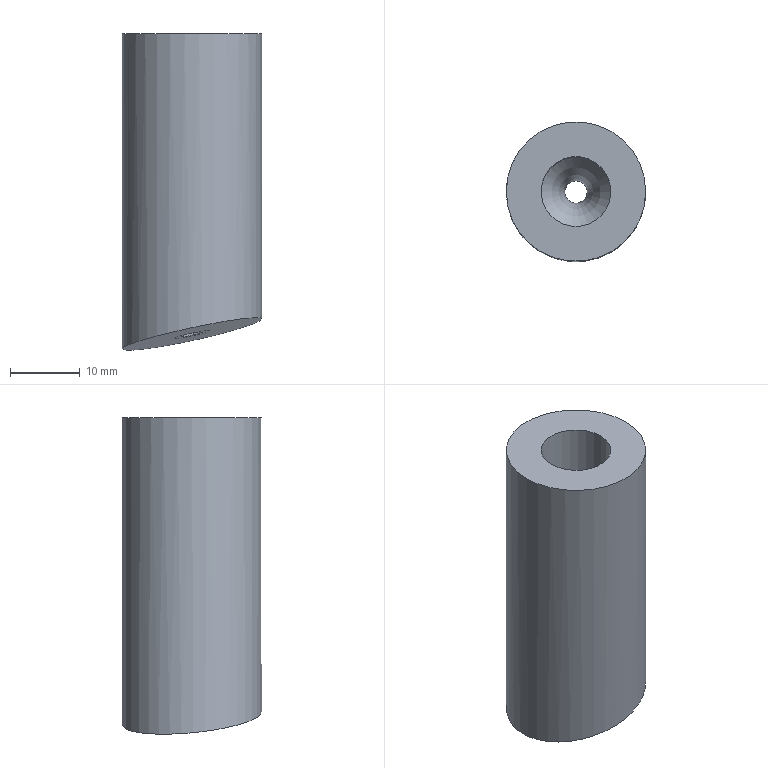Part | NX | features solid 2 | 1 solid | 7 faces | box 20 x 20 x 45.366 mm | volume 10880 mm3 | cylinder 3 | spline 2 | plane 1 | torus 1 | commonest cylinder face diameters 3.2 x1 10 x1 20 x1
STEP:
#1=CARTESIAN_POINT('',(379.199,-390.091,-10.));
#2=VERTEX_POINT('',#1);
#3=CARTESIAN_POINT('',(389.199,-390.091,-10.));
#4=DIRECTION('',(0.,0.,-1.));
#5=DIRECTION('',(-1.,0.,0.));
#6=AXIS2_PLACEMENT_3D('',#3,#4,#5);
#7=CIRCLE('',#6,10.);
#8=EDGE_CURVE('',#2,#2,#7,.T.);
#9=ORIENTED_EDGE('',*,*,#8,.F.);
#10=EDGE_LOOP('',(#9));
#11=FACE_BOUND('',#10,.T.);
#12=CARTESIAN_POINT('',(384.199,-390.091,-10.));
#13=VERTEX_POINT('',#12);
#14=CARTESIAN_POINT('',(389.199,-390.091,-10.));
#15=DIRECTION('',(0.,0.,-1.));
#16=DIRECTION('',(-1.,0.,0.));
#17=AXIS2_PLACEMENT_3D('',#14,#15,#16);
#18=CIRCLE('',#17,5.);
#19=EDGE_CURVE('',#13,#13,#18,.F.);
#20=ORIENTED_EDGE('',*,*,#19,.F.);
#21=EDGE_LOOP('',(#20));
#22=FACE_BOUND('',#21,.T.);
#23=CARTESIAN_POINT('',(389.199,-390.091,-10.));
#24=DIRECTION('',(0.,0.,-1.));
#25=DIRECTION('',(-1.,0.,0.));
#26=AXIS2_PLACEMENT_3D('',#23,#24,#25);
#27=PLANE('',#26);
#28=ADVANCED_FACE('',(#11,#22),#27,.F.);
#29=CARTESIAN_POINT('',(399.199,-390.091,-50.862));
#30=VERTEX_POINT('',#29);
#31=CARTESIAN_POINT('',(396.951,-398.053,-50.641));
#32=CARTESIAN_POINT('',(400.312,-390.059,-50.612));
#33=CARTESIAN_POINT('',(396.994,-382.26,-52.083));
#34=CARTESIAN_POINT('',(389.354,-379.042,-54.069));
#35=CARTESIAN_POINT('',(381.453,-382.122,-55.451));
#36=CARTESIAN_POINT('',(378.088,-390.11,-55.394));
#37=CARTESIAN_POINT('',(381.392,-397.916,-53.994));
#38=CARTESIAN_POINT('',(389.059,-401.144,-52.086));
#39=CARTESIAN_POINT('',(396.951,-398.053,-50.641));
#40=CARTESIAN_POINT('',(400.312,-390.059,-50.612));
#41=CARTESIAN_POINT('',(396.994,-382.26,-52.083));
#42=B_SPLINE_CURVE_WITH_KNOTS('',3,(#31,#32,#33,#34,#35,#36,#37,#38,#39,#40,#41),.UNSPECIFIED.,.T.,.F.,(1,1,1,1,1,1,1,1,1,1,1,1,1,1,1),(-0.02376,-0.01584,-0.007921,0.,0.007921,0.01584,0.02376,0.03168,0.03961,0.04753,0.05545,0.06337,0.07129,0.07921,0.08713),.UNSPECIFIED.);
#43=EDGE_CURVE('',#30,#30,#42,.T.);
#44=ORIENTED_EDGE('',*,*,#43,.T.);
#45=EDGE_LOOP('',(#44));
#46=FACE_BOUND('',#45,.T.);
#47=ORIENTED_EDGE('',*,*,#8,.T.);
#48=EDGE_LOOP('',(#47));
#49=FACE_BOUND('',#48,.T.);
#50=CARTESIAN_POINT('',(389.199,-390.091,-60.));
#51=DIRECTION('',(0.,0.,1.));
#52=DIRECTION('',(1.,0.,0.));
#53=AXIS2_PLACEMENT_3D('',#50,#51,#52);
#54=CYLINDRICAL_SURFACE('',#53,10.);
#55=ADVANCED_FACE('',(#46,#49),#54,.T.);
#56=CARTESIAN_POINT('',(384.199,-390.091,-40.705));
#57=VERTEX_POINT('',#56);
#58=CARTESIAN_POINT('',(389.199,-390.091,-40.705));
#59=DIRECTION('',(0.,0.,-1.));
#60=DIRECTION('',(-1.,0.,0.));
#61=AXIS2_PLACEMENT_3D('',#58,#59,#60);
#62=CIRCLE('',#61,5.);
#63=EDGE_CURVE('',#57,#57,#62,.F.);
#64=ORIENTED_EDGE('',*,*,#63,.F.);
#65=EDGE_LOOP('',(#64));
#66=FACE_BOUND('',#65,.T.);
#67=ORIENTED_EDGE('',*,*,#19,.T.);
#68=EDGE_LOOP('',(#67));
#69=FACE_BOUND('',#68,.T.);
#70=CARTESIAN_POINT('',(389.199,-390.091,20.));
#71=DIRECTION('',(0.,0.,-1.));
#72=DIRECTION('',(0.,-1.,0.));
#73=AXIS2_PLACEMENT_3D('',#70,#71,#72);
#74=CYLINDRICAL_SURFACE('',#73,5.);
#75=ADVANCED_FACE('',(#66,#69),#74,.F.);
#76=CARTESIAN_POINT('',(389.199,-388.491,-53.227));
#77=VERTEX_POINT('',#76);
#78=CARTESIAN_POINT('',(387.943,-388.833,-53.466));
#79=CARTESIAN_POINT('',(389.205,-388.322,-53.242));
#80=CARTESIAN_POINT('',(390.434,-388.827,-52.93));
#81=CARTESIAN_POINT('',(390.976,-390.067,-52.697));
#82=CARTESIAN_POINT('',(390.456,-391.35,-52.692));
#83=CARTESIAN_POINT('',(389.195,-391.86,-52.917));
#84=CARTESIAN_POINT('',(387.965,-391.358,-53.227));
#85=CARTESIAN_POINT('',(387.422,-390.118,-53.458));
#86=CARTESIAN_POINT('',(387.943,-388.833,-53.466));
#87=CARTESIAN_POINT('',(389.205,-388.322,-53.242));
#88=CARTESIAN_POINT('',(390.434,-388.827,-52.93));
#89=B_SPLINE_CURVE_WITH_KNOTS('',3,(#78,#79,#80,#81,#82,#83,#84,#85,#86,#87,#88),.UNSPECIFIED.,.T.,.F.,(1,1,1,1,1,1,1,1,1,1,1,1,1,1,1),(-0.003801,-0.002534,-0.001267,0.,0.001267,0.002534,0.003801,0.005068,0.006335,0.007602,0.008869,0.01014,0.0114,0.01267,0.01394),.UNSPECIFIED.);
#90=EDGE_CURVE('',#77,#77,#89,.T.);
#91=ORIENTED_EDGE('',*,*,#90,.T.);
#92=EDGE_LOOP('',(#91));
#93=FACE_BOUND('',#92,.T.);
#94=CARTESIAN_POINT('',(390.799,-390.091,-48.614));
#95=VERTEX_POINT('',#94);
#96=CARTESIAN_POINT('',(389.199,-390.091,-48.614));
#97=DIRECTION('',(0.,0.,1.));
#98=DIRECTION('',(1.,0.,0.));
#99=AXIS2_PLACEMENT_3D('',#96,#97,#98);
#100=CIRCLE('',#99,1.6);
#101=EDGE_CURVE('',#95,#95,#100,.F.);
#102=ORIENTED_EDGE('',*,*,#101,.F.);
#103=EDGE_LOOP('',(#102));
#104=FACE_BOUND('',#103,.T.);
#105=CARTESIAN_POINT('',(389.199,-390.091,-70.));
#106=DIRECTION('',(0.,0.,1.));
#107=DIRECTION('',(0.,1.,0.));
#108=AXIS2_PLACEMENT_3D('',#105,#106,#107);
#109=CYLINDRICAL_SURFACE('',#108,1.6);
#110=ADVANCED_FACE('',(#93,#104),#109,.F.);
#111=ORIENTED_EDGE('',*,*,#101,.T.);
#112=EDGE_LOOP('',(#111));
#113=FACE_BOUND('',#112,.T.);
#114=ORIENTED_EDGE('',*,*,#63,.T.);
#115=EDGE_LOOP('',(#114));
#116=FACE_BOUND('',#115,.T.);
#117=CARTESIAN_POINT('',(389.199,-390.091,-48.614));
#118=DIRECTION('',(0.,0.,1.));
#119=DIRECTION('',(1.,0.,0.));
#120=AXIS2_PLACEMENT_3D('',#117,#118,#119);
#121=TOROIDAL_SURFACE('',#120,12.5,10.9);
#122=ADVANCED_FACE('',(#113,#116),#121,.T.);
#123=CARTESIAN_POINT('',(391.151,-391.517,-52.525));
#124=VERTEX_POINT('',#123);
#125=CARTESIAN_POINT('',(387.237,-388.609,-53.637));
#126=VERTEX_POINT('',#125);
#127=CARTESIAN_POINT('',(391.151,-391.517,-52.525));
#128=CARTESIAN_POINT('',(390.742,-392.081,-52.562));
#129=CARTESIAN_POINT('',(389.562,-392.779,-52.753));
#130=CARTESIAN_POINT('',(387.554,-392.294,-53.228));
#131=CARTESIAN_POINT('',(386.527,-390.507,-53.612));
#132=CARTESIAN_POINT('',(386.83,-389.169,-53.672));
#133=CARTESIAN_POINT('',(387.237,-388.609,-53.637));
#134=B_SPLINE_CURVE_WITH_KNOTS('',3,(#127,#128,#129,#130,#131,#132,#133),.UNSPECIFIED.,.F.,.F.,(4,1,1,1,4),(0.,0.25,0.5,0.75,1.),.UNSPECIFIED.);
#135=EDGE_CURVE('',#124,#126,#134,.T.);
#136=ORIENTED_EDGE('',*,*,#135,.F.);
#137=CARTESIAN_POINT('',(387.237,-388.609,-53.637));
#138=CARTESIAN_POINT('',(387.646,-388.045,-53.602));
#139=CARTESIAN_POINT('',(388.826,-387.347,-53.414));
#140=CARTESIAN_POINT('',(390.834,-387.832,-52.935));
#141=CARTESIAN_POINT('',(391.86,-389.619,-52.546));
#142=CARTESIAN_POINT('',(391.557,-390.957,-52.489));
#143=CARTESIAN_POINT('',(391.151,-391.517,-52.525));
#144=B_SPLINE_CURVE_WITH_KNOTS('',3,(#137,#138,#139,#140,#141,#142,#143),.UNSPECIFIED.,.F.,.F.,(4,1,1,1,4),(0.,0.25,0.5,0.75,1.),.UNSPECIFIED.);
#145=EDGE_CURVE('',#126,#124,#144,.T.);
#146=ORIENTED_EDGE('',*,*,#145,.F.);
#147=EDGE_LOOP('',(#136,#146));
#148=FACE_BOUND('',#147,.T.);
#149=ORIENTED_EDGE('',*,*,#43,.F.);
#150=EDGE_LOOP('',(#149));
#151=FACE_BOUND('',#150,.T.);
#152=CARTESIAN_POINT('',(399.25,-399.794,-49.946));
#153=CARTESIAN_POINT('',(395.197,-399.98,-50.852));
#154=CARTESIAN_POINT('',(391.138,-400.164,-51.731));
#155=CARTESIAN_POINT('',(387.076,-400.345,-52.585));
#156=CARTESIAN_POINT('',(383.009,-400.524,-53.414));
#157=CARTESIAN_POINT('',(378.938,-400.701,-54.22));
#158=CARTESIAN_POINT('',(399.282,-395.73,-50.323));
#159=CARTESIAN_POINT('',(395.228,-395.913,-51.23));
#160=CARTESIAN_POINT('',(391.17,-396.095,-52.111));
#161=CARTESIAN_POINT('',(387.108,-396.274,-52.967));
#162=CARTESIAN_POINT('',(383.041,-396.451,-53.797));
#163=CARTESIAN_POINT('',(378.97,-396.626,-54.604));
#164=CARTESIAN_POINT('',(399.313,-391.664,-50.695));
#165=CARTESIAN_POINT('',(395.259,-391.846,-51.603));
#166=CARTESIAN_POINT('',(391.202,-392.025,-52.486));
#167=CARTESIAN_POINT('',(387.14,-392.203,-53.343));
#168=CARTESIAN_POINT('',(383.073,-392.378,-54.175));
#169=CARTESIAN_POINT('',(379.003,-392.551,-54.982));
#170=CARTESIAN_POINT('',(399.343,-387.598,-51.061));
#171=CARTESIAN_POINT('',(395.29,-387.777,-51.971));
#172=CARTESIAN_POINT('',(391.233,-387.955,-52.855));
#173=CARTESIAN_POINT('',(387.171,-388.13,-53.714));
#174=CARTESIAN_POINT('',(383.105,-388.304,-54.547));
#175=CARTESIAN_POINT('',(379.035,-388.475,-55.356));
#176=CARTESIAN_POINT('',(399.373,-383.531,-51.422));
#177=CARTESIAN_POINT('',(395.321,-383.708,-52.334));
#178=CARTESIAN_POINT('',(391.264,-383.884,-53.22));
#179=CARTESIAN_POINT('',(387.202,-384.058,-54.08));
#180=CARTESIAN_POINT('',(383.136,-384.229,-54.914));
#181=CARTESIAN_POINT('',(379.066,-384.398,-55.724));
#182=CARTESIAN_POINT('',(399.403,-379.463,-51.778));
#183=CARTESIAN_POINT('',(395.35,-379.639,-52.692));
#184=CARTESIAN_POINT('',(391.294,-379.812,-53.579));
#185=CARTESIAN_POINT('',(387.233,-379.984,-54.44));
#186=CARTESIAN_POINT('',(383.167,-380.153,-55.276));
#187=CARTESIAN_POINT('',(379.097,-380.321,-56.087));
#188=B_SPLINE_SURFACE_WITH_KNOTS('',5,5,((#152,#153,#154,#155,#156,#157),(#158,#159,#160,#161,#162,#163),(#164,#165,#166,#167,#168,#169),(#170,#171,#172,#173,#174,#175),(#176,#177,#178,#179,#180,#181),(#182,#183,#184,#185,#186,#187)),.UNSPECIFIED.,.F.,.F.,.F.,(6,6),(6,6),(0.1757,0.9201),(0.1016,0.3573),.PIECEWISE_BEZIER_KNOTS.);
#189=ADVANCED_FACE('',(#148,#151),#188,.F.);
#190=ORIENTED_EDGE('',*,*,#135,.T.);
#191=ORIENTED_EDGE('',*,*,#145,.T.);
#192=EDGE_LOOP('',(#190,#191));
#193=FACE_BOUND('',#192,.T.);
#194=ORIENTED_EDGE('',*,*,#90,.F.);
#195=EDGE_LOOP('',(#194));
#196=FACE_BOUND('',#195,.T.);
#197=CARTESIAN_POINT('',(391.698,-392.573,-52.307));
#198=CARTESIAN_POINT('',(390.673,-392.618,-52.527));
#199=CARTESIAN_POINT('',(389.648,-392.663,-52.745));
#200=CARTESIAN_POINT('',(388.623,-392.708,-52.961));
#201=CARTESIAN_POINT('',(387.597,-392.752,-53.176));
#202=CARTESIAN_POINT('',(386.571,-392.797,-53.389));
#203=CARTESIAN_POINT('',(391.706,-391.536,-52.402));
#204=CARTESIAN_POINT('',(390.681,-391.581,-52.622));
#205=CARTESIAN_POINT('',(389.656,-391.626,-52.84));
#206=CARTESIAN_POINT('',(388.631,-391.671,-53.056));
#207=CARTESIAN_POINT('',(387.605,-391.715,-53.271));
#208=CARTESIAN_POINT('',(386.579,-391.76,-53.484));
#209=CARTESIAN_POINT('',(391.714,-390.5,-52.497));
#210=CARTESIAN_POINT('',(390.689,-390.545,-52.716));
#211=CARTESIAN_POINT('',(389.664,-390.589,-52.935));
#212=CARTESIAN_POINT('',(388.639,-390.634,-53.151));
#213=CARTESIAN_POINT('',(387.613,-390.679,-53.366));
#214=CARTESIAN_POINT('',(386.587,-390.723,-53.579));
#215=CARTESIAN_POINT('',(391.722,-389.463,-52.591));
#216=CARTESIAN_POINT('',(390.697,-389.508,-52.811));
#217=CARTESIAN_POINT('',(389.672,-389.553,-53.029));
#218=CARTESIAN_POINT('',(388.647,-389.597,-53.245));
#219=CARTESIAN_POINT('',(387.621,-389.642,-53.46));
#220=CARTESIAN_POINT('',(386.595,-389.686,-53.674));
#221=CARTESIAN_POINT('',(391.73,-388.427,-52.684));
#222=CARTESIAN_POINT('',(390.705,-388.471,-52.904));
#223=CARTESIAN_POINT('',(389.68,-388.516,-53.123));
#224=CARTESIAN_POINT('',(388.654,-388.56,-53.339));
#225=CARTESIAN_POINT('',(387.629,-388.605,-53.554));
#226=CARTESIAN_POINT('',(386.603,-388.649,-53.768));
#227=CARTESIAN_POINT('',(391.738,-387.39,-52.778));
#228=CARTESIAN_POINT('',(390.713,-387.435,-52.998));
#229=CARTESIAN_POINT('',(389.688,-387.479,-53.216));
#230=CARTESIAN_POINT('',(388.662,-387.523,-53.433));
#231=CARTESIAN_POINT('',(387.637,-387.567,-53.648));
#232=CARTESIAN_POINT('',(386.611,-387.611,-53.862));
#233=B_SPLINE_SURFACE_WITH_KNOTS('',5,5,((#197,#198,#199,#200,#201,#202),(#203,#204,#205,#206,#207,#208),(#209,#210,#211,#212,#213,#214),(#215,#216,#217,#218,#219,#220),(#221,#222,#223,#224,#225,#226),(#227,#228,#229,#230,#231,#232)),.UNSPECIFIED.,.F.,.F.,.F.,(6,6),(6,6),(0.4525,0.6421),(0.1975,0.262),.PIECEWISE_BEZIER_KNOTS.);
#234=ADVANCED_FACE('',(#193,#196),#233,.F.);
#235=CLOSED_SHELL('',(#28,#55,#75,#110,#122,#189,#234));
#236=MANIFOLD_SOLID_BREP('',#235);
#237=(LENGTH_UNIT()NAMED_UNIT(*)SI_UNIT(.MILLI.,.METRE.));
#238=UNCERTAINTY_MEASURE_WITH_UNIT(LENGTH_MEASURE(0.0508),#237,'','');
#239=(NAMED_UNIT(*)PLANE_ANGLE_UNIT()SI_UNIT($,.RADIAN.));
#240=(NAMED_UNIT(*)SI_UNIT($,.STERADIAN.)SOLID_ANGLE_UNIT());
#241=(GEOMETRIC_REPRESENTATION_CONTEXT(3)GLOBAL_UNCERTAINTY_ASSIGNED_CONTEXT((#238))GLOBAL_UNIT_ASSIGNED_CONTEXT((#237,#239,#240))REPRESENTATION_CONTEXT('',''));
#242=ADVANCED_BREP_SHAPE_REPRESENTATION('',(#236),#241);